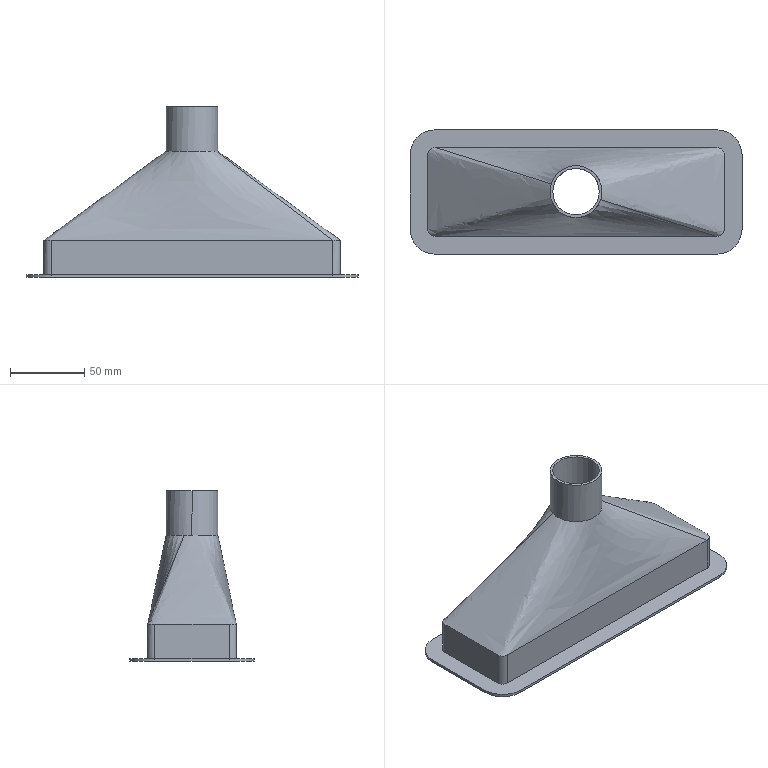Part | SolidWorks | features ICE 2, Blend 1, Extrusion 1, Shell 1 | 1 solid | 35 faces | box 224 x 84 x 115 mm | volume 101490 mm3 | cylinder 16 | plane 15 | spline 4 | commonest cylinder face diameters 6.4 x4 10 x4 34 x4 31.4 x2 35 x2